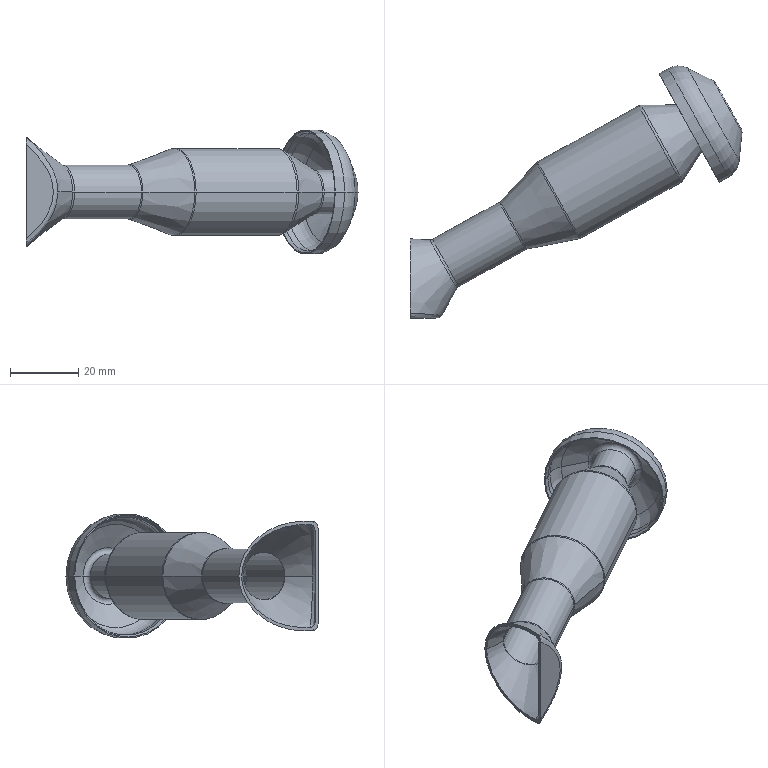Part | STEP file | Completa.sldasm-Part-31_Valor predeterminado | 1 solid | 59 faces | box 97.324 x 73.886 x 36.376 mm | volume 6808 mm3 | torus 18 | cone 18 | cylinder 16 | plane 5 | spline 2 | commonest cylinder face diameters 11.219 x2 12.819 x2 14.267 x2 15.867 x2 24.058 x2 25.658 x2